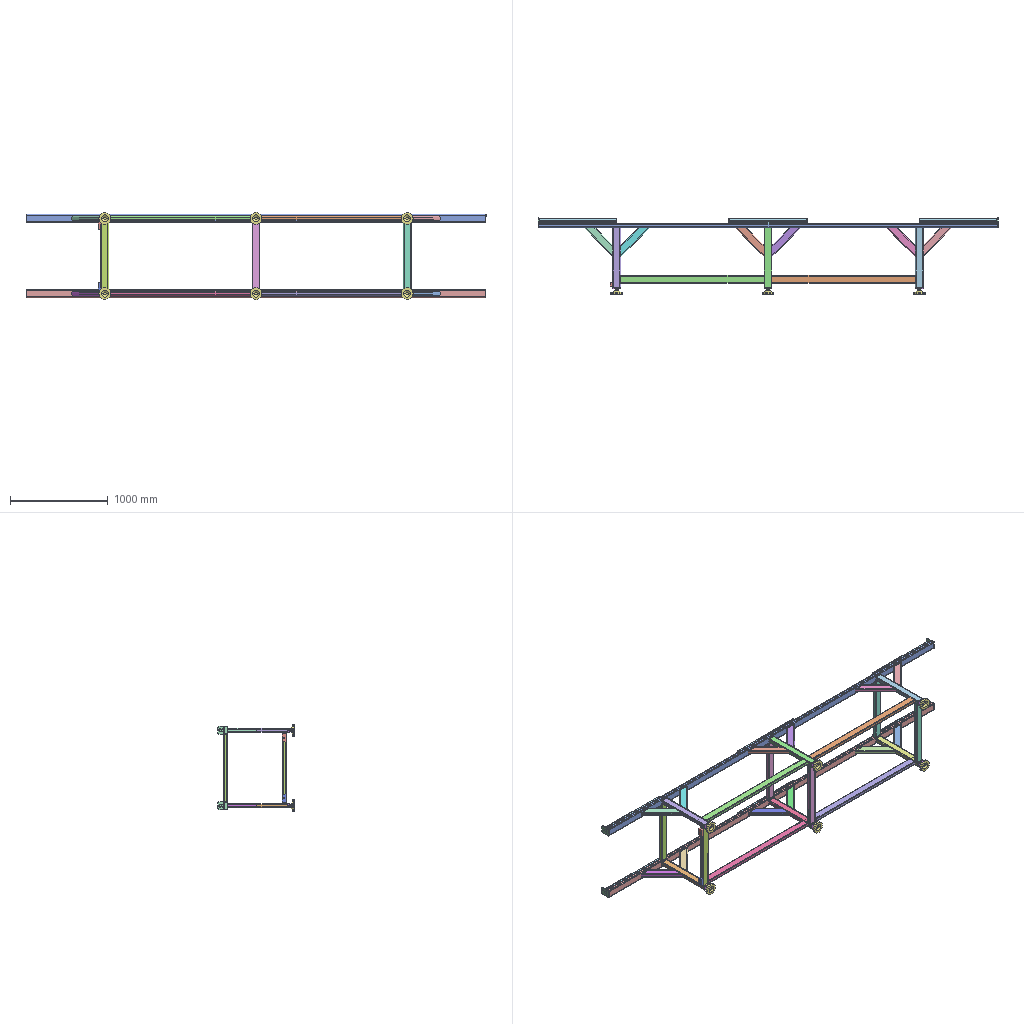Assembly | SolidWorks | 6 different items | 24 placed | box 4716 x 780 x 892 mm
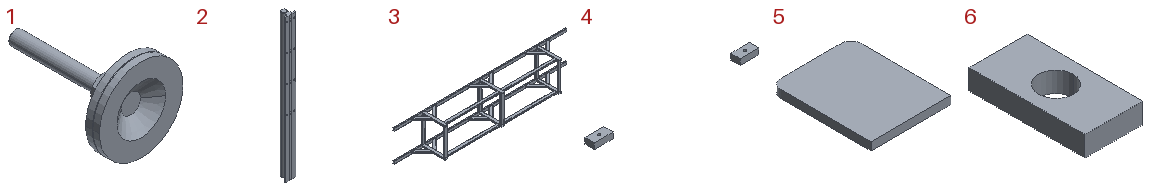Parts list (item | quantity | size | volume | features):
1 | x6 | 120 x 181 x 120 mm | 289918 mm3 | features ICE 2, RevCut 2, Chamfer 1, Revolution 1
2 | x6 | 60 x 52 x 800 mm | 1150861 mm3 | features RevCut 2, Chamfer 1, CurvePattern 1, Extrusion 1, ICE 1, MirrorPattern 1
3 | x1 | 4700 x 650 x 854 mm | 23333323 mm3 | features WeldCornerFeat 3, 3DProfileFeature 1, MoveCopyBody 1, WeldMemberFeat 1, WeldmentFeature 1
4 | x1 | 700 x 40 x 25 mm | 155914 mm3 | features Extrusion 1, HoleWzd 1
5 | x4 | 80 x 100 x 8 mm | 63657 mm3 | features Extrusion 1, Fillet 1
6 | x6 | 40 x 80 x 14 mm | 38467 mm3 | features Extrusion 1
Mates (type | each side: item.copy, entity, surface, feature):
Coincident | 3.1 face plane SOLIDWORKS GB/T 6728-1986 rectangular hollow steel profile | 2.1 face plane Boss-Extrude1
Coincident | 3.1 face plane SOLIDWORKS GB/T 6728-1986 rectangular hollow steel profile | 2.1 face plane Boss-Extrude2
Width | 2.1 face plane Boss-Extrude1 | 2.1 face plane Boss-Extrude1 | 3.1 face plane SOLIDWORKS GB/T 6728-1986 rectangular hollow steel profile | 3.1 face plane SOLIDWORKS GB/T 6728-1986 rectangular hollow steel profile
Width | 2.2 face plane Boss-Extrude1 | 2.2 face plane Boss-Extrude1 | 3.1 face plane SOLIDWORKS GB/T 6728-1986 rectangular hollow steel profile | 3.1 face plane SOLIDWORKS GB/T 6728-1986 rectangular hollow steel profile
Coincident | 3.1 face plane SOLIDWORKS GB/T 6728-1986 rectangular hollow steel profile | 2.2 face plane Boss-Extrude1
Coincident | 2.2 face plane Boss-Extrude2 | 2.1 face plane Boss-Extrude2
Coincident | 1.1 face plane Boss-Extrude2 | 6.1 face plane Boss-Extrude1
Concentric | 1.1 face cylinder Revolve1 | 6.1 face cylinder Boss-Extrude1
Coincident | 3.1 face plane SOLIDWORKS GB/T 6728-1986 rectangular hollow steel profile | 6.1 face plane Boss-Extrude1 | 3 times
Coincident | 3.1 face plane SOLIDWORKS GB/T 6728-1986 rectangular hollow steel profile | 5.1 face plane Boss-Extrude1 | 3 times
Coincident | 3.1 face plane SOLIDWORKS GB/T 6728-1986 rectangular hollow steel profile | 5.2 face plane Boss-Extrude1 | 3 times
Coincident | 3.1 face plane SOLIDWORKS GB/T 6728-1986 rectangular hollow steel profile | 5.3 face plane Boss-Extrude1 | 3 times
Coincident | 3.1 face plane SOLIDWORKS GB/T 6728-1986 rectangular hollow steel profile | 5.4 face plane Boss-Extrude1 | 3 times
Coincident | 3.1 face plane SOLIDWORKS GB/T 6728-1986 rectangular hollow steel profile | 4.1 face plane Boss-Extrude1 | 2 times
Width | 3.1 face plane SOLIDWORKS GB/T 6728-1986 rectangular hollow steel profile | 3.1 face plane SOLIDWORKS GB/T 6728-1986 rectangular hollow steel profile | 4.1 face plane Boss-Extrude1 | 4.1 face plane Boss-Extrude1